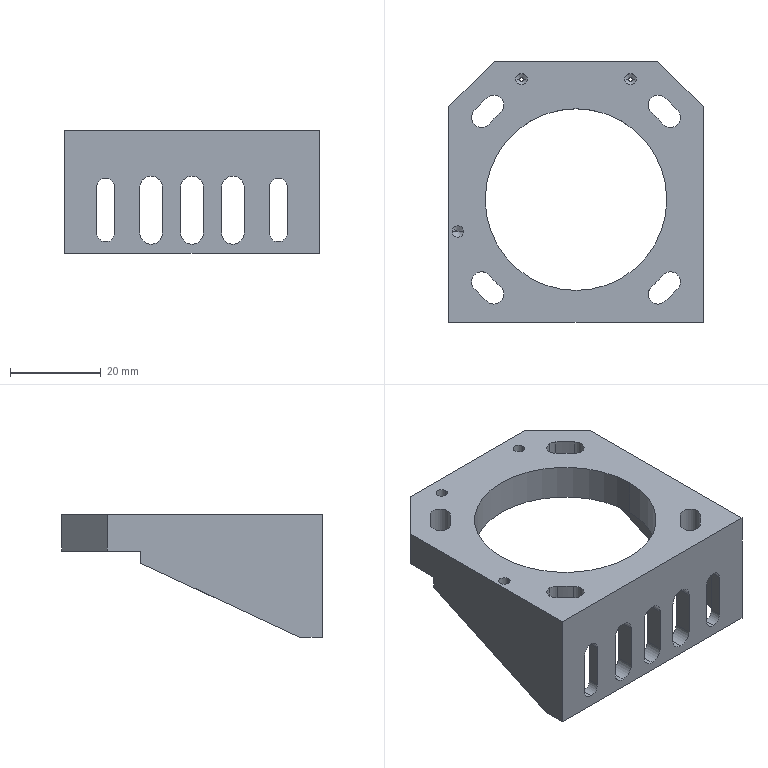NC program | NX | posted with a generic post | part box 56 x 57.4 x 27 mm
Lines 338 to 1845 of 23725:
(FLOOR_WALL_1 , TOOL : D10C)
N668 T10 M6
N670 G54
N672 G17 G0 G90 X34.7 Y4.041 B0. C0. S2500 M3
N674 G43 Z30. H10
N676 Z0.9
N678 G94 G1 Z-0.1 F1000.
N680 X29.2 Y0.866
N682 G3 X28.7 Y0. R1.
N684 G1 Y-18. F2500.
N686 X18.7 Y-28.
N688 X16.4
N690 Y-19.9
N692 X-21.1
N694 Y-16.612
N696 G3 X-19.6 Y-13. R5.1
N698 G1 Y13.
N700 G3 X-21.1 Y16.612 R5.1
N702 G1 Y19.9
N704 X16.4
N706 Y28.
N708 X18.7
N710 X28.7 Y18.
N712 Y0.
N714 X21.7
N716 Y-15.101
N718 X21.594 Y-15.207
N720 G3 X16.4 Y-12.9 R7.
N722 G1 X-12.6
N724 Y12.9
N726 X16.4
N728 G3 X21.594 Y15.207 R7.
N730 G1 X21.7 Y15.101
N732 Y0.
N734 X14.7
N736 Y-5.9
N738 X-5.6
N740 Y5.9
N742 X14.7
N744 Y0.
N746 X10.2
N748 Y-1.4
N750 X-1.1
N752 Y1.4
N754 X10.2
N756 Y0.
N758 G3 X10.7 Y-0.866 R1.
N760 G1 Z0.9
N762 G0 X34.7 Y4.041 Z0.8
N764 G1 Z-0.2 F1000.
N766 X29.2 Y0.866
N768 G3 X28.7 Y0. R1.
N770 G1 Y-18. F2500.
N772 X18.7 Y-28.
N774 X16.4
N776 Y-19.9
N778 X-21.1
N780 Y-16.612
N782 G3 X-19.6 Y-13. R5.1
N784 G1 Y13.
N786 G3 X-21.1 Y16.612 R5.1
N788 G1 Y19.9
N790 X16.4
N792 Y28.
N794 X18.7
N796 X28.7 Y18.
N798 Y0.
N800 X21.7
N802 Y-15.101
N804 X21.594 Y-15.207
N806 G3 X16.4 Y-12.9 R7.
N808 G1 X-12.6
N810 Y12.9
N812 X16.4
N814 G3 X21.594 Y15.207 R7.
N816 G1 X21.7 Y15.101
N818 Y0.
N820 X14.7
N822 Y-5.9
N824 X-5.6
N826 Y5.9
N828 X14.7
N830 Y0.
N832 X10.2
N834 Y-1.4
N836 X-1.1
N838 Y1.4
N840 X10.2
N842 Y0.
N844 G3 X10.7 Y-0.866 R1.
N846 G1 Z0.8
N848 G0 X34.7 Y4.041 Z0.7
N850 G1 Z-0.3 F1000.
N852 X29.2 Y0.866
N854 G3 X28.7 Y0. R1.
N856 G1 Y-18. F2500.
N858 X18.7 Y-28.
N860 X16.4
N862 Y-19.9
N864 X-21.1
N866 Y-16.612
N868 G3 X-19.6 Y-13. R5.1
N870 G1 Y13.
N872 G3 X-21.1 Y16.612 R5.1
N874 G1 Y19.9
N876 X16.4
N878 Y28.
N880 X18.7
N882 X28.7 Y18.
N884 Y0.
N886 X21.7
N888 Y-15.101
N890 X21.594 Y-15.207
N892 G3 X16.4 Y-12.9 R7.
N894 G1 X-12.6
N896 Y12.9
N898 X16.4
N900 G3 X21.594 Y15.207 R7.
N902 G1 X21.7 Y15.101
N904 Y0.
N906 X14.7
N908 Y-5.9
N910 X-5.6
N912 Y5.9
N914 X14.7
N916 Y0.
N918 X10.2
N920 Y-1.4
N922 X-1.1
N924 Y1.4
N926 X10.2
N928 Y0.
N930 G3 X10.7 Y-0.866 R1.
N932 G1 Z0.7
N934 G0 X34.7 Y4.041 Z0.6
N936 G1 Z-0.4 F1000.
N938 X29.2 Y0.866
N940 G3 X28.7 Y0. R1.
N942 G1 Y-18. F2500.
N944 X18.7 Y-28.
N946 X16.4
N948 Y-19.9
N950 X-21.1
N952 Y-16.612
N954 G3 X-19.6 Y-13. R5.1
N956 G1 Y13.
N958 G3 X-21.1 Y16.612 R5.1
N960 G1 Y19.9
N962 X16.4
N964 Y28.
N966 X18.7
N968 X28.7 Y18.
N970 Y0.
N972 X21.7
N974 Y-15.101
N976 X21.594 Y-15.207
N978 G3 X16.4 Y-12.9 R7.
N980 G1 X-12.6
N982 Y12.9
N984 X16.4
N986 G3 X21.594 Y15.207 R7.
N988 G1 X21.7 Y15.101
N990 Y0.
N992 X14.7
N994 Y-5.9
N996 X-5.6
N998 Y5.9
N1000 X14.7
N1002 Y0.
N1004 X10.2
N1006 Y-1.4
N1008 X-1.1
N1010 Y1.4
N1012 X10.2
N1014 Y0.
N1016 G3 X10.7 Y-0.866 R1.
N1018 G1 Z0.6
N1020 G0 X34.7 Y4.041 Z0.5
N1022 G1 Z-0.5 F1000.
N1024 X29.2 Y0.866
N1026 G3 X28.7 Y0. R1.
N1028 G1 Y-18. F2500.
N1030 X18.7 Y-28.
N1032 X16.4
N1034 Y-19.9
N1036 X-21.1
N1038 Y-16.612
N1040 G3 X-19.6 Y-13. R5.1
N1042 G1 Y13.
N1044 G3 X-21.1 Y16.612 R5.1
N1046 G1 Y19.9
N1048 X16.4
N1050 Y28.
N1052 X18.7
N1054 X28.7 Y18.
N1056 Y0.
N1058 X21.7
N1060 Y-15.101
N1062 X21.594 Y-15.207
N1064 G3 X16.4 Y-12.9 R7.
N1066 G1 X-12.6
N1068 Y12.9
N1070 X16.4
N1072 G3 X21.594 Y15.207 R7.
N1074 G1 X21.7 Y15.101
N1076 Y0.
N1078 X14.7
N1080 Y-5.9
N1082 X-5.6
N1084 Y5.9
N1086 X14.7
N1088 Y0.
N1090 X10.2
N1092 Y-1.4
N1094 X-1.1
N1096 Y1.4
N1098 X10.2
N1100 Y0.
N1102 G3 X10.7 Y-0.866 R1.
N1104 G1 Z0.5
N1106 G0 X34.7 Y4.041 Z0.4
N1108 G1 Z-0.6 F1000.
N1110 X29.2 Y0.866
N1112 G3 X28.7 Y0. R1.
N1114 G1 Y-18. F2500.
N1116 X18.7 Y-28.
N1118 X16.4
N1120 Y-19.9
N1122 X-21.1
N1124 Y-16.612
N1126 G3 X-19.6 Y-13. R5.1
N1128 G1 Y13.
N1130 G3 X-21.1 Y16.612 R5.1
N1132 G1 Y19.9
N1134 X16.4
N1136 Y28.
N1138 X18.7
N1140 X28.7 Y18.
N1142 Y0.
N1144 X21.7
N1146 Y-15.101
N1148 X21.594 Y-15.207
N1150 G3 X16.4 Y-12.9 R7.
N1152 G1 X-12.6
N1154 Y12.9
N1156 X16.4
N1158 G3 X21.594 Y15.207 R7.
N1160 G1 X21.7 Y15.101
N1162 Y0.
N1164 X14.7
N1166 Y-5.9
N1168 X-5.6
N1170 Y5.9
N1172 X14.7
N1174 Y0.
N1176 X10.2
N1178 Y-1.4
N1180 X-1.1
N1182 Y1.4
N1184 X10.2
N1186 Y0.
N1188 G3 X10.7 Y-0.866 R1.
N1190 G1 Z0.4
N1192 G0 X34.7 Y4.041 Z0.3
N1194 G1 Z-0.7 F1000.
N1196 X29.2 Y0.866
N1198 G3 X28.7 Y0. R1.
N1200 G1 Y-18. F2500.
N1202 X18.7 Y-28.
N1204 X16.4
N1206 Y-19.9
N1208 X-21.1
N1210 Y-16.612
N1212 G3 X-19.6 Y-13. R5.1
N1214 G1 Y13.
N1216 G3 X-21.1 Y16.612 R5.1
N1218 G1 Y19.9
N1220 X16.4
N1222 Y28.
N1224 X18.7
N1226 X28.7 Y18.
N1228 Y0.
N1230 X21.7
N1232 Y-15.101
N1234 X21.594 Y-15.207
N1236 G3 X16.4 Y-12.9 R7.
N1238 G1 X-12.6
N1240 Y12.9
N1242 X16.4
N1244 G3 X21.594 Y15.207 R7.
N1246 G1 X21.7 Y15.101
N1248 Y0.
N1250 X14.7
N1252 Y-5.9
N1254 X-5.6
N1256 Y5.9
N1258 X14.7
N1260 Y0.
N1262 X10.2
N1264 Y-1.4
N1266 X-1.1
N1268 Y1.4
N1270 X10.2
N1272 Y0.
N1274 G3 X10.7 Y-0.866 R1.
N1276 G1 Z0.3
N1278 G0 X34.7 Y4.041 Z0.2
N1280 G1 Z-0.8 F1000.
N1282 X29.2 Y0.866
N1284 G3 X28.7 Y0. R1.
N1286 G1 Y-18. F2500.
N1288 X18.7 Y-28.
N1290 X16.4
N1292 Y-19.9
N1294 X-21.1
N1296 Y-16.612
N1298 G3 X-19.6 Y-13. R5.1
N1300 G1 Y13.
N1302 G3 X-21.1 Y16.612 R5.1
N1304 G1 Y19.9
N1306 X16.4
N1308 Y28.
N1310 X18.7
N1312 X28.7 Y18.
N1314 Y0.
N1316 X21.7
N1318 Y-15.101
N1320 X21.594 Y-15.207
N1322 G3 X16.4 Y-12.9 R7.
N1324 G1 X-12.6
N1326 Y12.9
N1328 X16.4
N1330 G3 X21.594 Y15.207 R7.
N1332 G1 X21.7 Y15.101
N1334 Y0.
N1336 X14.7
N1338 Y-5.9
N1340 X-5.6
N1342 Y5.9
N1344 X14.7
N1346 Y0.
N1348 X10.2
N1350 Y-1.4
N1352 X-1.1
N1354 Y1.4
N1356 X10.2
N1358 Y0.
N1360 G3 X10.7 Y-0.866 R1.
N1362 G1 Z0.2
N1364 G0 X34.7 Y4.041 Z0.1
N1366 G1 Z-0.9 F1000.
N1368 X29.2 Y0.866
N1370 G3 X28.7 Y0. R1.
N1372 G1 Y-18. F2500.
N1374 X18.7 Y-28.
N1376 X16.4
N1378 Y-19.9
N1380 X-21.1
N1382 Y-16.612
N1384 G3 X-19.6 Y-13. R5.1
N1386 G1 Y13.
N1388 G3 X-21.1 Y16.612 R5.1
N1390 G1 Y19.9
N1392 X16.4
N1394 Y28.
N1396 X18.7
N1398 X28.7 Y18.
N1400 Y0.
N1402 X21.7
N1404 Y-15.101
N1406 X21.594 Y-15.207
N1408 G3 X16.4 Y-12.9 R7.
N1410 G1 X-12.6
N1412 Y12.9
N1414 X16.4
N1416 G3 X21.594 Y15.207 R7.
N1418 G1 X21.7 Y15.101
N1420 Y0.
N1422 X14.7
N1424 Y-5.9
N1426 X-5.6
N1428 Y5.9
N1430 X14.7
N1432 Y0.
N1434 X10.2
N1436 Y-1.4
N1438 X-1.1
N1440 Y1.4
N1442 X10.2
N1444 Y0.
N1446 G3 X10.7 Y-0.866 R1.
N1448 G1 Z0.1
N1450 G0 X34.7 Y4.041 Z0.
N1452 G1 Z-1. F1000.
N1454 X29.2 Y0.866
N1456 G3 X28.7 Y0. R1.
N1458 G1 Y-18. F2500.
N1460 X18.7 Y-28.
N1462 X16.4
N1464 Y-19.9
N1466 X-21.1
N1468 Y-16.612
N1470 G3 X-19.6 Y-13. R5.1
N1472 G1 Y13.
N1474 G3 X-21.1 Y16.612 R5.1
N1476 G1 Y19.9
N1478 X16.4
N1480 Y28.
N1482 X18.7
N1484 X28.7 Y18.
N1486 Y0.
N1488 X21.7
N1490 Y-15.101
N1492 X21.594 Y-15.207
N1494 G3 X16.4 Y-12.9 R7.
N1496 G1 X-12.6
N1498 Y12.9
N1500 X16.4
N1502 G3 X21.594 Y15.207 R7.
N1504 G1 X21.7 Y15.101
N1506 Y0.
N1508 X14.7
N1510 Y-5.9
N1512 X-5.6
N1514 Y5.9
N1516 X14.7
N1518 Y0.
N1520 X10.2
N1522 Y-1.4
N1524 X-1.1
N1526 Y1.4
N1528 X10.2
N1530 Y0.
N1532 G3 X10.7 Y-0.866 R1.
N1534 G1 Z0.
N1536 G0 X34.7 Y4.041 Z-0.1
N1538 G1 Z-1.1 F1000.
N1540 X29.2 Y0.866
N1542 G3 X28.7 Y0. R1.
N1544 G1 Y-18. F2500.
N1546 X18.7 Y-28.
N1548 X16.4
N1550 Y-19.9
N1552 X-21.1
N1554 Y-16.612
N1556 G3 X-19.6 Y-13. R5.1
N1558 G1 Y13.
N1560 G3 X-21.1 Y16.612 R5.1
N1562 G1 Y19.9
N1564 X16.4
N1566 Y28.
N1568 X18.7
N1570 X28.7 Y18.
N1572 Y0.
N1574 X21.7
N1576 Y-15.101
N1578 X21.594 Y-15.207
N1580 G3 X16.4 Y-12.9 R7.
N1582 G1 X-12.6
N1584 Y12.9
N1586 X16.4
N1588 G3 X21.594 Y15.207 R7.
N1590 G1 X21.7 Y15.101
N1592 Y0.
N1594 X14.7
N1596 Y-5.9
N1598 X-5.6
N1600 Y5.9
N1602 X14.7
N1604 Y0.
N1606 X10.2
N1608 Y-1.4
N1610 X-1.1
N1612 Y1.4
N1614 X10.2
N1616 Y0.
N1618 G3 X10.7 Y-0.866 R1.
N1620 G1 Z-0.1
N1622 G0 X34.7 Y4.041 Z-0.2
N1624 G1 Z-1.2 F1000.
N1626 X29.2 Y0.866
N1628 G3 X28.7 Y0. R1.
N1630 G1 Y-18. F2500.
N1632 X18.7 Y-28.
N1634 X16.4
N1636 Y-19.9
N1638 X-21.1
N1640 Y-16.612
N1642 G3 X-19.6 Y-13. R5.1
N1644 G1 Y13.
N1646 G3 X-21.1 Y16.612 R5.1
N1648 G1 Y19.9
N1650 X16.4
N1652 Y28.
N1654 X18.7
N1656 X28.7 Y18.
N1658 Y0.
N1660 X21.7
N1662 Y-15.101
N1664 X21.594 Y-15.207
N1666 G3 X16.4 Y-12.9 R7.
N1668 G1 X-12.6
N1670 Y12.9
N1672 X16.4
N1674 G3 X21.594 Y15.207 R7.
N1676 G1 X21.7 Y15.101
N1678 Y0.
N1680 X14.7
N1682 Y-5.9
N1684 X-5.6
N1686 Y5.9
N1688 X14.7
N1690 Y0.
N1692 X10.2
N1694 Y-1.4
N1696 X-1.1
N1698 Y1.4
N1700 X10.2
N1702 Y0.
N1704 G3 X10.7 Y-0.866 R1.
N1706 G1 Z-0.2
N1708 G0 X34.7 Y4.041 Z-0.3
N1710 G1 Z-1.3 F1000.
N1712 X29.2 Y0.866
N1714 G3 X28.7 Y0. R1.
N1716 G1 Y-18. F2500.
N1718 X18.7 Y-28.
N1720 X16.4
N1722 Y-19.9
N1724 X-21.1
N1726 Y-16.612
N1728 G3 X-19.6 Y-13. R5.1
N1730 G1 Y13.
N1732 G3 X-21.1 Y16.612 R5.1
N1734 G1 Y19.9
N1736 X16.4
N1738 Y28.
N1740 X18.7
N1742 X28.7 Y18.
N1744 Y0.
N1746 X21.7
N1748 Y-15.101
N1750 X21.594 Y-15.207
N1752 G3 X16.4 Y-12.9 R7.
N1754 G1 X-12.6
N1756 Y12.9
N1758 X16.4
N1760 G3 X21.594 Y15.207 R7.
N1762 G1 X21.7 Y15.101
N1764 Y0.
N1766 X14.7
N1768 Y-5.9
N1770 X-5.6
N1772 Y5.9
N1774 X14.7
N1776 Y0.
N1778 X10.2
N1780 Y-1.4
N1782 X-1.1
N1784 Y1.4
N1786 X10.2
N1788 Y0.
N1790 G3 X10.7 Y-0.866 R1.
N1792 G1 Z-0.3
N1794 G0 X34.7 Y4.041 Z-0.4
N1796 G1 Z-1.4 F1000.
N1798 X29.2 Y0.866
N1800 G3 X28.7 Y0. R1.
N1802 G1 Y-18. F2500.
N1804 X18.7 Y-28.
N1806 X16.4
N1808 Y-19.9
N1810 X-21.1
N1812 Y-16.612
N1814 G3 X-19.6 Y-13. R5.1
N1816 G1 Y13.
N1818 G3 X-21.1 Y16.612 R5.1
N1820 G1 Y19.9
N1822 X16.4
N1824 Y28.
N1826 X18.7
N1828 X28.7 Y18.
N1830 Y0.
N1832 X21.7
N1834 Y-15.101
N1836 X21.594 Y-15.207
N1838 G3 X16.4 Y-12.9 R7.
N1840 G1 X-12.6
N1842 Y12.9
N1844 X16.4
N1846 G3 X21.594 Y15.207 R7.
N1848 G1 X21.7 Y15.101
N1850 Y0.
N1852 X14.7
N1854 Y-5.9
N1856 X-5.6
N1858 Y5.9
N1860 X14.7
N1862 Y0.
N1864 X10.2
N1866 Y-1.4
N1868 X-1.1
N1870 Y1.4
N1872 X10.2
N1874 Y0.
N1876 G3 X10.7 Y-0.866 R1.
N1878 G1 Z-0.4
N1880 G0 X34.7 Y4.041 Z-0.5
N1882 G1 Z-1.5 F1000.
N1884 X29.2 Y0.866
N1886 G3 X28.7 Y0. R1.
N1888 G1 Y-18. F2500.
N1890 X18.7 Y-28.
N1892 X16.4
N1894 Y-19.9
N1896 X-21.1
N1898 Y-16.612
N1900 G3 X-19.6 Y-13. R5.1
N1902 G1 Y13.
N1904 G3 X-21.1 Y16.612 R5.1
N1906 G1 Y19.9
N1908 X16.4
N1910 Y28.
N1912 X18.7
N1914 X28.7 Y18.
N1916 Y0.
N1918 X21.7
N1920 Y-15.101
N1922 X21.594 Y-15.207
N1924 G3 X16.4 Y-12.9 R7.
N1926 G1 X-12.6
N1928 Y12.9
N1930 X16.4
N1932 G3 X21.594 Y15.207 R7.
N1934 G1 X21.7 Y15.101
N1936 Y0.
N1938 X14.7
N1940 Y-5.9
N1942 X-5.6
N1944 Y5.9
N1946 X14.7
N1948 Y0.
N1950 X10.2
N1952 Y-1.4
N1954 X-1.1
N1956 Y1.4
N1958 X10.2
N1960 Y0.
N1962 G3 X10.7 Y-0.866 R1.
N1964 G1 Z-0.5
N1966 G0 X34.7 Y4.041 Z-0.6
N1968 G1 Z-1.6 F1000.
N1970 X29.2 Y0.866
N1972 G3 X28.7 Y0. R1.
N1974 G1 Y-18. F2500.
N1976 X18.7 Y-28.
N1978 X16.4
N1980 Y-19.9
N1982 X-21.1
N1984 Y-16.612
N1986 G3 X-19.6 Y-13. R5.1
N1988 G1 Y13.
N1990 G3 X-21.1 Y16.612 R5.1
N1992 G1 Y19.9
N1994 X16.4
N1996 Y28.
N1998 X18.7
N2000 X28.7 Y18.
N2002 Y0.
N2004 X21.7
N2006 Y-15.101
N2008 X21.594 Y-15.207
N2010 G3 X16.4 Y-12.9 R7.
N2012 G1 X-12.6
N2014 Y12.9
N2016 X16.4
N2018 G3 X21.594 Y15.207 R7.
N2020 G1 X21.7 Y15.101
N2022 Y0.
N2024 X14.7
N2026 Y-5.9
N2028 X-5.6
N2030 Y5.9
N2032 X14.7
N2034 Y0.
N2036 X10.2
N2038 Y-1.4
N2040 X-1.1
N2042 Y1.4
N2044 X10.2
N2046 Y0.
N2048 G3 X10.7 Y-0.866 R1.
N2050 G1 Z-0.6
N2052 G0 X34.7 Y4.041 Z-0.7
N2054 G1 Z-1.7 F1000.
N2056 X29.2 Y0.866
N2058 G3 X28.7 Y0. R1.
N2060 G1 Y-18. F2500.
N2062 X18.7 Y-28.
N2064 X16.4
N2066 Y-19.9
N2068 X-21.1
N2070 Y-16.612
N2072 G3 X-19.6 Y-13. R5.1
N2074 G1 Y13.
N2076 G3 X-21.1 Y16.612 R5.1
N2078 G1 Y19.9
N2080 X16.4
N2082 Y28.
N2084 X18.7
N2086 X28.7 Y18.
N2088 Y0.
N2090 X21.7
N2092 Y-15.101
N2094 X21.594 Y-15.207
N2096 G3 X16.4 Y-12.9 R7.
N2098 G1 X-12.6
N2100 Y12.9
N2102 X16.4
N2104 G3 X21.594 Y15.207 R7.
N2106 G1 X21.7 Y15.101
N2108 Y0.
N2110 X14.7
N2112 Y-5.9
N2114 X-5.6
N2116 Y5.9
N2118 X14.7
N2120 Y0.
N2122 X10.2
N2124 Y-1.4
N2126 X-1.1
N2128 Y1.4
N2130 X10.2
N2132 Y0.
N2134 G3 X10.7 Y-0.866 R1.
N2136 G1 Z-0.7
N2138 G0 X34.7 Y4.041 Z-0.8
N2140 G1 Z-1.8 F1000.
N2142 X29.2 Y0.866
N2144 G3 X28.7 Y0. R1.
N2146 G1 Y-18. F2500.
N2148 X18.7 Y-28.
N2150 X16.4
N2152 Y-19.9
N2154 X-21.1
N2156 Y-16.612
N2158 G3 X-19.6 Y-13. R5.1
N2160 G1 Y13.
N2162 G3 X-21.1 Y16.612 R5.1
N2164 G1 Y19.9
N2166 X16.4
N2168 Y28.
N2170 X18.7
N2172 X28.7 Y18.
N2174 Y0.
N2176 X21.7
N2178 Y-15.101
N2180 X21.594 Y-15.207
N2182 G3 X16.4 Y-12.9 R7.
N2184 G1 X-12.6
N2186 Y12.9
N2188 X16.4
N2190 G3 X21.594 Y15.207 R7.
N2192 G1 X21.7 Y15.101
N2194 Y0.
N2196 X14.7
N2198 Y-5.9
N2200 X-5.6
N2202 Y5.9
N2204 X14.7
N2206 Y0.
N2208 X10.2
N2210 Y-1.4
N2212 X-1.1
N2214 Y1.4
N2216 X10.2
N2218 Y0.
N2220 G3 X10.7 Y-0.866 R1.
N2222 G1 Z-0.8
N2224 G0 X34.7 Y4.041 Z-0.9
N2226 G1 Z-1.9 F1000.
N2228 X29.2 Y0.866
N2230 G3 X28.7 Y0. R1.
N2232 G1 Y-18. F2500.
N2234 X18.7 Y-28.
N2236 X16.4
N2238 Y-19.9
N2240 X-21.1
N2242 Y-16.612
N2244 G3 X-19.6 Y-13. R5.1
N2246 G1 Y13.
N2248 G3 X-21.1 Y16.612 R5.1
N2250 G1 Y19.9
N2252 X16.4
N2254 Y28.
N2256 X18.7
N2258 X28.7 Y18.
N2260 Y0.
N2262 X21.7
N2264 Y-15.101
N2266 X21.594 Y-15.207
N2268 G3 X16.4 Y-12.9 R7.
N2270 G1 X-12.6
N2272 Y12.9
N2274 X16.4
N2276 G3 X21.594 Y15.207 R7.
N2278 G1 X21.7 Y15.101
N2280 Y0.
N2282 X14.7
N2284 Y-5.9
N2286 X-5.6
N2288 Y5.9
N2290 X14.7
N2292 Y0.
N2294 X10.2
N2296 Y-1.4
N2298 X-1.1
N2300 Y1.4
N2302 X10.2
N2304 Y0.
N2306 G3 X10.7 Y-0.866 R1.
N2308 G1 Z-0.9
N2310 G0 X34.7 Y4.041 Z-1.
N2312 G1 Z-2. F1000.
N2314 X29.2 Y0.866
N2316 G3 X28.7 Y0. R1.
N2318 G1 Y-18. F2500.
N2320 X18.7 Y-28.
N2322 X16.4
N2324 Y-19.9
N2326 X-21.1
N2328 Y-16.612
N2330 G3 X-19.6 Y-13. R5.1
N2332 G1 Y13.
N2334 G3 X-21.1 Y16.612 R5.1
N2336 G1 Y19.9
N2338 X16.4
N2340 Y28.
N2342 X18.7
N2344 X28.7 Y18.
N2346 Y0.
N2348 X21.7
N2350 Y-15.101
N2352 X21.594 Y-15.207
N2354 G3 X16.4 Y-12.9 R7.
N2356 G1 X-12.6
N2358 Y12.9
N2360 X16.4
N2362 G3 X21.594 Y15.207 R7.
N2364 G1 X21.7 Y15.101
N2366 Y0.
N2368 X14.7
N2370 Y-5.9
N2372 X-5.6
N2374 Y5.9
N2376 X14.7
N2378 Y0.
N2380 X10.2
N2382 Y-1.4
N2384 X-1.1
N2386 Y1.4
N2388 X10.2
N2390 Y0.
N2392 G3 X10.7 Y-0.866 R1.
N2394 G1 Z-1.
N2396 G0 X34.7 Y4.041 Z-1.1
N2398 G1 Z-2.1 F1000.
N2400 X29.2 Y0.866
N2402 G3 X28.7 Y0. R1.
N2404 G1 Y-18. F2500.
N2406 X18.7 Y-28.
N2408 X16.4
N2410 Y-19.9
N2412 X-21.1
N2414 Y-16.612
N2416 G3 X-19.6 Y-13. R5.1
N2418 G1 Y13.
N2420 G3 X-21.1 Y16.612 R5.1
N2422 G1 Y19.9
N2424 X16.4
N2426 Y28.
N2428 X18.7
N2430 X28.7 Y18.
N2432 Y0.
N2434 X21.7
N2436 Y-15.101
N2438 X21.594 Y-15.207
N2440 G3 X16.4 Y-12.9 R7.
N2442 G1 X-12.6
N2444 Y12.9
N2446 X16.4
N2448 G3 X21.594 Y15.207 R7.
N2450 G1 X21.7 Y15.101
N2452 Y0.
N2454 X14.7
N2456 Y-5.9
N2458 X-5.6
N2460 Y5.9
N2462 X14.7
N2464 Y0.
N2466 X10.2
N2468 Y-1.4
N2470 X-1.1
N2472 Y1.4
N2474 X10.2
N2476 Y0.
N2478 G3 X10.7 Y-0.866 R1.
N2480 G1 Z-1.1
N2482 G0 X34.7 Y4.041 Z-1.2
N2484 G1 Z-2.2 F1000.
N2486 X29.2 Y0.866
N2488 G3 X28.7 Y0. R1.
N2490 G1 Y-18. F2500.
N2492 X18.7 Y-28.
N2494 X16.4
N2496 Y-19.9
N2498 X-21.1
N2500 Y-16.612
N2502 G3 X-19.6 Y-13. R5.1
N2504 G1 Y13.
N2506 G3 X-21.1 Y16.612 R5.1
N2508 G1 Y19.9
N2510 X16.4
N2512 Y28.
N2514 X18.7
N2516 X28.7 Y18.
N2518 Y0.
N2520 X21.7
N2522 Y-15.101
N2524 X21.594 Y-15.207
N2526 G3 X16.4 Y-12.9 R7.
N2528 G1 X-12.6
N2530 Y12.9
N2532 X16.4
N2534 G3 X21.594 Y15.207 R7.
N2536 G1 X21.7 Y15.101
N2538 Y0.
N2540 X14.7
N2542 Y-5.9
N2544 X-5.6
N2546 Y5.9
N2548 X14.7
N2550 Y0.
N2552 X10.2
N2554 Y-1.4
N2556 X-1.1
N2558 Y1.4
N2560 X10.2
N2562 Y0.
N2564 G3 X10.7 Y-0.866 R1.
N2566 G1 Z-1.2
N2568 G0 X34.7 Y4.041 Z-1.3
N2570 G1 Z-2.3 F1000.
N2572 X29.2 Y0.866
N2574 G3 X28.7 Y0. R1.
N2576 G1 Y-18. F2500.
N2578 X18.7 Y-28.
N2580 X16.4
N2582 Y-19.9
N2584 X-21.1
N2586 Y-16.612
N2588 G3 X-19.6 Y-13. R5.1
N2590 G1 Y13.
N2592 G3 X-21.1 Y16.612 R5.1
N2594 G1 Y19.9
N2596 X16.4
N2598 Y28.
N2600 X18.7
N2602 X28.7 Y18.
N2604 Y0.
N2606 X21.7
N2608 Y-15.101
N2610 X21.594 Y-15.207
N2612 G3 X16.4 Y-12.9 R7.
N2614 G1 X-12.6
N2616 Y12.9
N2618 X16.4
N2620 G3 X21.594 Y15.207 R7.
N2622 G1 X21.7 Y15.101
N2624 Y0.
N2626 X14.7
N2628 Y-5.9
N2630 X-5.6
N2632 Y5.9
N2634 X14.7
N2636 Y0.
N2638 X10.2
N2640 Y-1.4
N2642 X-1.1
N2644 Y1.4
N2646 X10.2
N2648 Y0.
N2650 G3 X10.7 Y-0.866 R1.
N2652 G1 Z-1.3
N2654 G0 X34.7 Y4.041 Z-1.4
N2656 G1 Z-2.4 F1000.
N2658 X29.2 Y0.866
N2660 G3 X28.7 Y0. R1.
N2662 G1 Y-18. F2500.
N2664 X18.7 Y-28.
N2666 X16.4
N2668 Y-19.9
N2670 X-21.1
N2672 Y-16.612
N2674 G3 X-19.6 Y-13. R5.1
N2676 G1 Y13.
N2678 G3 X-21.1 Y16.612 R5.1
N2680 G1 Y19.9
N2682 X16.4
N2684 Y28.
N2686 X18.7
N2688 X28.7 Y18.
N2690 Y0.
N2692 X21.7
N2694 Y-15.101
N2696 X21.594 Y-15.207
N2698 G3 X16.4 Y-12.9 R7.
N2700 G1 X-12.6
N2702 Y12.9
N2704 X16.4
N2706 G3 X21.594 Y15.207 R7.
N2708 G1 X21.7 Y15.101
N2710 Y0.
N2712 X14.7
N2714 Y-5.9
N2716 X-5.6
N2718 Y5.9
N2720 X14.7
N2722 Y0.
N2724 X10.2
N2726 Y-1.4
N2728 X-1.1
N2730 Y1.4
N2732 X10.2
N2734 Y0.
N2736 G3 X10.7 Y-0.866 R1.
N2738 G1 Z-1.4
N2740 G0 X34.7 Y4.041 Z-1.5
N2742 G1 Z-2.5 F1000.
N2744 X29.2 Y0.866
N2746 G3 X28.7 Y0. R1.
N2748 G1 Y-18. F2500.
N2750 X18.7 Y-28.
N2752 X16.4
N2754 Y-19.9
N2756 X-21.1
N2758 Y-16.612
N2760 G3 X-19.6 Y-13. R5.1
N2762 G1 Y13.
N2764 G3 X-21.1 Y16.612 R5.1
N2766 G1 Y19.9
N2768 X16.4
N2770 Y28.
N2772 X18.7
N2774 X28.7 Y18.
N2776 Y0.
N2778 X21.7
N2780 Y-15.101
N2782 X21.594 Y-15.207
N2784 G3 X16.4 Y-12.9 R7.
N2786 G1 X-12.6
N2788 Y12.9
N2790 X16.4
N2792 G3 X21.594 Y15.207 R7.
N2794 G1 X21.7 Y15.101
N2796 Y0.
N2798 X14.7
N2800 Y-5.9
N2802 X-5.6
N2804 Y5.9
N2806 X14.7
N2808 Y0.
N2810 X10.2
N2812 Y-1.4
N2814 X-1.1
N2816 Y1.4
N2818 X10.2
N2820 Y0.
N2822 G3 X10.7 Y-0.866 R1.
N2824 G1 Z-1.5
N2826 G0 X34.7 Y4.041 Z-1.6
N2828 G1 Z-2.6 F1000.
N2830 X29.2 Y0.866
N2832 G3 X28.7 Y0. R1.
N2834 G1 Y-18. F2500.
N2836 X18.7 Y-28.
N2838 X16.4
N2840 Y-19.9
N2842 X-21.1
N2844 Y-16.612
N2846 G3 X-19.6 Y-13. R5.1
N2848 G1 Y13.
N2850 G3 X-21.1 Y16.612 R5.1
N2852 G1 Y19.9
N2854 X16.4
N2856 Y28.
N2858 X18.7
N2860 X28.7 Y18.
N2862 Y0.
N2864 X21.7
N2866 Y-15.101
N2868 X21.594 Y-15.207
N2870 G3 X16.4 Y-12.9 R7.
N2872 G1 X-12.6
N2874 Y12.9
N2876 X16.4
N2878 G3 X21.594 Y15.207 R7.
N2880 G1 X21.7 Y15.101
N2882 Y0.
N2884 X14.7
N2886 Y-5.9
N2888 X-5.6
N2890 Y5.9
N2892 X14.7
N2894 Y0.
N2896 X10.2
N2898 Y-1.4
N2900 X-1.1
N2902 Y1.4
N2904 X10.2
N2906 Y0.
N2908 G3 X10.7 Y-0.866 R1.
N2910 G1 Z-1.6
N2912 G0 X34.7 Y4.041 Z-1.7
N2914 G1 Z-2.7 F1000.
N2916 X29.2 Y0.866
N2918 G3 X28.7 Y0. R1.
N2920 G1 Y-18. F2500.
N2922 X18.7 Y-28.
N2924 X16.4
N2926 Y-19.9
N2928 X-21.1
N2930 Y-16.612
N2932 G3 X-19.6 Y-13. R5.1
N2934 G1 Y13.
N2936 G3 X-21.1 Y16.612 R5.1
N2938 G1 Y19.9
N2940 X16.4
N2942 Y28.
N2944 X18.7
N2946 X28.7 Y18.
N2948 Y0.
N2950 X21.7
N2952 Y-15.101
N2954 X21.594 Y-15.207
N2956 G3 X16.4 Y-12.9 R7.
N2958 G1 X-12.6
N2960 Y12.9
N2962 X16.4
N2964 G3 X21.594 Y15.207 R7.
N2966 G1 X21.7 Y15.101
N2968 Y0.
N2970 X14.7
N2972 Y-5.9
N2974 X-5.6
N2976 Y5.9
N2978 X14.7
N2980 Y0.
N2982 X10.2
N2984 Y-1.4
N2986 X-1.1
N2988 Y1.4
N2990 X10.2
N2992 Y0.
N2994 G3 X10.7 Y-0.866 R1.
N2996 G1 Z-1.7
N2998 G0 X34.7 Y4.041 Z-1.8
N3000 G1 Z-2.8 F1000.
N3002 X29.2 Y0.866
N3004 G3 X28.7 Y0. R1.
N3006 G1 Y-18. F2500.
N3008 X18.7 Y-28.
N3010 X16.4
N3012 Y-19.9
N3014 X-21.1
N3016 Y-16.612
N3018 G3 X-19.6 Y-13. R5.1
N3020 G1 Y13.
N3022 G3 X-21.1 Y16.612 R5.1
N3024 G1 Y19.9
N3026 X16.4
N3028 Y28.
N3030 X18.7
N3032 X28.7 Y18.
N3034 Y0.
N3036 X21.7
N3038 Y-15.101
N3040 X21.594 Y-15.207
N3042 G3 X16.4 Y-12.9 R7.
N3044 G1 X-12.6
N3046 Y12.9
N3048 X16.4
N3050 G3 X21.594 Y15.207 R7.
N3052 G1 X21.7 Y15.101
N3054 Y0.
N3056 X14.7
N3058 Y-5.9
N3060 X-5.6
N3062 Y5.9
N3064 X14.7
N3066 Y0.
N3068 X10.2
N3070 Y-1.4
N3072 X-1.1
N3074 Y1.4
N3076 X10.2
N3078 Y0.
N3080 G3 X10.7 Y-0.866 R1.
N3082 G1 Z-1.8
N3084 G0 X34.7 Y4.041 Z-1.9
N3086 G1 Z-2.9 F1000.
N3088 X29.2 Y0.866
N3090 G3 X28.7 Y0. R1.
N3092 G1 Y-18. F2500.
N3094 X18.7 Y-28.
N3096 X16.4
N3098 Y-19.9
N3100 X-21.1
N3102 Y-16.612
N3104 G3 X-19.6 Y-13. R5.1
N3106 G1 Y13.
N3108 G3 X-21.1 Y16.612 R5.1
N3110 G1 Y19.9
N3112 X16.4
N3114 Y28.
N3116 X18.7
N3118 X28.7 Y18.
N3120 Y0.
N3122 X21.7
N3124 Y-15.101
N3126 X21.594 Y-15.207
N3128 G3 X16.4 Y-12.9 R7.
N3130 G1 X-12.6
N3132 Y12.9
N3134 X16.4
N3136 G3 X21.594 Y15.207 R7.
N3138 G1 X21.7 Y15.101
N3140 Y0.
N3142 X14.7
N3144 Y-5.9
N3146 X-5.6
N3148 Y5.9
N3150 X14.7
N3152 Y0.
N3154 X10.2
N3156 Y-1.4
N3158 X-1.1
N3160 Y1.4
N3162 X10.2
N3164 Y0.
N3166 G3 X10.7 Y-0.866 R1.
N3168 G1 Z-1.9
N3170 G0 X34.7 Y4.041 Z-2.
N3172 G1 Z-3. F1000.
N3174 X29.2 Y0.866
N3176 G3 X28.7 Y0. R1.
N3178 G1 Y-18. F2500.
N3180 X18.7 Y-28.
N3182 X16.4
N3184 Y-19.9
N3186 X-21.1
N3188 Y-16.612
N3190 G3 X-19.6 Y-13. R5.1
N3192 G1 Y13.
N3194 G3 X-21.1 Y16.612 R5.1
N3196 G1 Y19.9
N3198 X16.4
N3200 Y28.
N3202 X18.7
N3204 X28.7 Y18.
N3206 Y0.
N3208 X21.7
N3210 Y-15.101
N3212 X21.594 Y-15.207
N3214 G3 X16.4 Y-12.9 R7.
N3216 G1 X-12.6
N3218 Y12.9
N3220 X16.4
N3222 G3 X21.594 Y15.207 R7.
N3224 G1 X21.7 Y15.101
N3226 Y0.
N3228 X14.7
N3230 Y-5.9
N3232 X-5.6
N3234 Y5.9
N3236 X14.7
N3238 Y0.
N3240 X10.2
N3242 Y-1.4
N3244 X-1.1
N3246 Y1.4
N3248 X10.2
N3250 Y0.
N3252 G3 X10.7 Y-0.866 R1.
N3254 G1 Z-2.
N3256 G0 X34.7 Y4.041 Z-2.1
N3258 G1 Z-3.1 F1000.
N3260 X29.2 Y0.866
N3262 G3 X28.7 Y0. R1.
N3264 G1 Y-18. F2500.
N3266 X18.7 Y-28.
N3268 X16.4
N3270 Y-19.9
N3272 X-21.1
N3274 Y-16.612
N3276 G3 X-19.6 Y-13. R5.1
N3278 G1 Y13.
N3280 G3 X-21.1 Y16.612 R5.1
N3282 G1 Y19.9
N3284 X16.4
N3286 Y28.
N3288 X18.7
N3290 X28.7 Y18.
N3292 Y0.
N3294 X21.7
N3296 Y-15.101
N3298 X21.594 Y-15.207
N3300 G3 X16.4 Y-12.9 R7.
N3302 G1 X-12.6
N3304 Y12.9
N3306 X16.4
N3308 G3 X21.594 Y15.207 R7.
N3310 G1 X21.7 Y15.101
N3312 Y0.
N3314 X14.7
N3316 Y-5.9
N3318 X-5.6
N3320 Y5.9
N3322 X14.7
N3324 Y0.
N3326 X10.2
N3328 Y-1.4
N3330 X-1.1
N3332 Y1.4
N3334 X10.2
N3336 Y0.
N3338 G3 X10.7 Y-0.866 R1.
N3340 G1 Z-2.1
N3342 G0 X34.7 Y4.041 Z-2.2
N3344 G1 Z-3.2 F1000.
N3346 X29.2 Y0.866
N3348 G3 X28.7 Y0. R1.
N3350 G1 Y-18. F2500.
N3352 X18.7 Y-28.
N3354 X16.4
N3356 Y-19.9
N3358 X-21.1
N3360 Y-16.612
N3362 G3 X-19.6 Y-13. R5.1
N3364 G1 Y13.
N3366 G3 X-21.1 Y16.612 R5.1
N3368 G1 Y19.9
N3370 X16.4
N3372 Y28.
N3374 X18.7
N3376 X28.7 Y18.
N3378 Y0.
N3380 X21.7
N3382 Y-15.101
N3384 X21.594 Y-15.207
N3386 G3 X16.4 Y-12.9 R7.
N3388 G1 X-12.6
N3390 Y12.9
N3392 X16.4
N3394 G3 X21.594 Y15.207 R7.
N3396 G1 X21.7 Y15.101
N3398 Y0.
N3400 X14.7
N3402 Y-5.9
N3404 X-5.6
N3406 Y5.9
N3408 X14.7
N3410 Y0.
N3412 X10.2
N3414 Y-1.4
N3416 X-1.1
N3418 Y1.4
N3420 X10.2
N3422 Y0.
N3424 G3 X10.7 Y-0.866 R1.
N3426 G1 Z-2.2
N3428 G0 X34.7 Y4.041 Z-2.3
N3430 G1 Z-3.3 F1000.
N3432 X29.2 Y0.866
N3434 G3 X28.7 Y0. R1.
N3436 G1 Y-18. F2500.
N3438 X18.7 Y-28.
N3440 X16.4
N3442 Y-19.9
N3444 X-21.1
N3446 Y-16.612
N3448 G3 X-19.6 Y-13. R5.1
N3450 G1 Y13.
N3452 G3 X-21.1 Y16.612 R5.1
N3454 G1 Y19.9
N3456 X16.4
N3458 Y28.
N3460 X18.7
N3462 X28.7 Y18.
N3464 Y0.
N3466 X21.7
N3468 Y-15.101
N3470 X21.594 Y-15.207
N3472 G3 X16.4 Y-12.9 R7.
N3474 G1 X-12.6
N3476 Y12.9
N3478 X16.4
N3480 G3 X21.594 Y15.207 R7.
N3482 G1 X21.7 Y15.101
N3484 Y0.
N3486 X14.7
N3488 Y-5.9
N3490 X-5.6
N3492 Y5.9
N3494 X14.7
N3496 Y0.
N3498 X10.2
N3500 Y-1.4
N3502 X-1.1
N3504 Y1.4
N3506 X10.2
N3508 Y0.
N3510 G3 X10.7 Y-0.866 R1.
N3512 G1 Z-2.3
N3514 G0 X34.7 Y4.041 Z-2.4
N3516 G1 Z-3.4 F1000.
N3518 X29.2 Y0.866
N3520 G3 X28.7 Y0. R1.
N3522 G1 Y-18. F2500.
N3524 X18.7 Y-28.
N3526 X16.4
N3528 Y-19.9
N3530 X-21.1
N3532 Y-16.612
N3534 G3 X-19.6 Y-13. R5.1
N3536 G1 Y13.
N3538 G3 X-21.1 Y16.612 R5.1
N3540 G1 Y19.9
N3542 X16.4
N3544 Y28.
N3546 X18.7
N3548 X28.7 Y18.
N3550 Y0.
N3552 X21.7
N3554 Y-15.101
N3556 X21.594 Y-15.207
N3558 G3 X16.4 Y-12.9 R7.
N3560 G1 X-12.6
N3562 Y12.9
N3564 X16.4
N3566 G3 X21.594 Y15.207 R7.
N3568 G1 X21.7 Y15.101
N3570 Y0.
N3572 X14.7
N3574 Y-5.9
N3576 X-5.6
N3578 Y5.9
N3580 X14.7
N3582 Y0.
N3584 X10.2
N3586 Y-1.4
N3588 X-1.1
N3590 Y1.4
N3592 X10.2
N3594 Y0.
N3596 G3 X10.7 Y-0.866 R1.
N3598 G1 Z-2.4
N3600 G0 X34.7 Y4.041 Z-2.5
N3602 G1 Z-3.5 F1000.
N3604 X29.2 Y0.866
N3606 G3 X28.7 Y0. R1.
N3608 G1 Y-18. F2500.
N3610 X18.7 Y-28.
N3612 X16.4
N3614 Y-19.9
N3616 X-21.1
N3618 Y-16.612
N3620 G3 X-19.6 Y-13. R5.1
N3622 G1 Y13.
N3624 G3 X-21.1 Y16.612 R5.1
N3626 G1 Y19.9
N3628 X16.4
N3630 Y28.
N3632 X18.7
N3634 X28.7 Y18.
N3636 Y0.
N3638 X21.7
N3640 Y-15.101
N3642 X21.594 Y-15.207
N3644 G3 X16.4 Y-12.9 R7.
N3646 G1 X-12.6
N3648 Y12.9
N3650 X16.4
N3652 G3 X21.594 Y15.207 R7.
N3654 G1 X21.7 Y15.101
N3656 Y0.
N3658 X14.7
N3660 Y-5.9
N3662 X-5.6
N3664 Y5.9
N3666 X14.7
N3668 Y0.
N3670 X10.2
N3672 Y-1.4
N3674 X-1.1
N3676 Y1.4